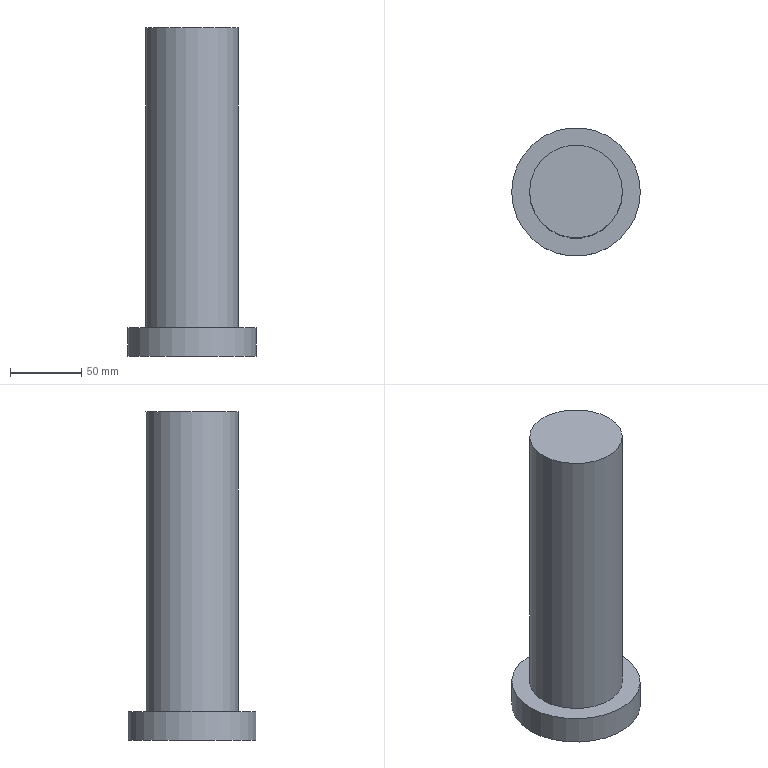Part | NX | features 平衡千斤顶缸销 2 | 1 solid | 5 faces | box 90 x 90 x 230 mm | volume 824079 mm3 | plane 3 | cylinder 2 | commonest cylinder face diameters 65 x1 90 x1
STEP:
#1=CARTESIAN_POINT('',(32.5,0.,210.));
#2=VERTEX_POINT('',#1);
#3=CARTESIAN_POINT('',(0.,0.,210.));
#4=DIRECTION('',(0.,0.,1.));
#5=DIRECTION('',(1.,0.,0.));
#6=AXIS2_PLACEMENT_3D('',#3,#4,#5);
#7=CIRCLE('',#6,32.5);
#8=EDGE_CURVE('',#2,#2,#7,.T.);
#9=ORIENTED_EDGE('',*,*,#8,.F.);
#10=EDGE_LOOP('',(#9));
#11=FACE_BOUND('',#10,.T.);
#12=CARTESIAN_POINT('',(-32.5,0.,0.));
#13=VERTEX_POINT('',#12);
#14=CARTESIAN_POINT('',(0.,0.,0.));
#15=DIRECTION('',(0.,0.,-1.));
#16=DIRECTION('',(-1.,0.,0.));
#17=AXIS2_PLACEMENT_3D('',#14,#15,#16);
#18=CIRCLE('',#17,32.5);
#19=EDGE_CURVE('',#13,#13,#18,.T.);
#20=ORIENTED_EDGE('',*,*,#19,.F.);
#21=EDGE_LOOP('',(#20));
#22=FACE_BOUND('',#21,.T.);
#23=CARTESIAN_POINT('',(0.,0.,210.));
#24=DIRECTION('',(0.,0.,-1.));
#25=DIRECTION('',(-1.,0.,0.));
#26=AXIS2_PLACEMENT_3D('',#23,#24,#25);
#27=CYLINDRICAL_SURFACE('',#26,32.5);
#28=ADVANCED_FACE('',(#11,#22),#27,.T.);
#29=ORIENTED_EDGE('',*,*,#8,.T.);
#30=EDGE_LOOP('',(#29));
#31=FACE_BOUND('',#30,.T.);
#32=CARTESIAN_POINT('',(0.,0.,210.));
#33=DIRECTION('',(0.,0.,1.));
#34=DIRECTION('',(1.,0.,0.));
#35=AXIS2_PLACEMENT_3D('',#32,#33,#34);
#36=PLANE('',#35);
#37=ADVANCED_FACE('',(#31),#36,.T.);
#38=CARTESIAN_POINT('',(-45.,0.,0.));
#39=VERTEX_POINT('',#38);
#40=CARTESIAN_POINT('',(0.,0.,0.));
#41=DIRECTION('',(0.,0.,-1.));
#42=DIRECTION('',(-1.,0.,0.));
#43=AXIS2_PLACEMENT_3D('',#40,#41,#42);
#44=CIRCLE('',#43,45.);
#45=EDGE_CURVE('',#39,#39,#44,.T.);
#46=ORIENTED_EDGE('',*,*,#45,.F.);
#47=EDGE_LOOP('',(#46));
#48=FACE_BOUND('',#47,.T.);
#49=ORIENTED_EDGE('',*,*,#19,.T.);
#50=EDGE_LOOP('',(#49));
#51=FACE_BOUND('',#50,.T.);
#52=CARTESIAN_POINT('',(0.,0.,0.));
#53=DIRECTION('',(0.,0.,-1.));
#54=DIRECTION('',(-1.,0.,0.));
#55=AXIS2_PLACEMENT_3D('',#52,#53,#54);
#56=PLANE('',#55);
#57=ADVANCED_FACE('',(#48,#51),#56,.F.);
#58=CARTESIAN_POINT('',(-45.,0.,-20.));
#59=VERTEX_POINT('',#58);
#60=CARTESIAN_POINT('',(0.,0.,-20.));
#61=DIRECTION('',(0.,0.,-1.));
#62=DIRECTION('',(-1.,0.,0.));
#63=AXIS2_PLACEMENT_3D('',#60,#61,#62);
#64=CIRCLE('',#63,45.);
#65=EDGE_CURVE('',#59,#59,#64,.T.);
#66=ORIENTED_EDGE('',*,*,#65,.F.);
#67=EDGE_LOOP('',(#66));
#68=FACE_BOUND('',#67,.T.);
#69=ORIENTED_EDGE('',*,*,#45,.T.);
#70=EDGE_LOOP('',(#69));
#71=FACE_BOUND('',#70,.T.);
#72=CARTESIAN_POINT('',(0.,0.,-20.));
#73=DIRECTION('',(0.,0.,1.));
#74=DIRECTION('',(1.,0.,0.));
#75=AXIS2_PLACEMENT_3D('',#72,#73,#74);
#76=CYLINDRICAL_SURFACE('',#75,45.);
#77=ADVANCED_FACE('',(#68,#71),#76,.T.);
#78=ORIENTED_EDGE('',*,*,#65,.T.);
#79=EDGE_LOOP('',(#78));
#80=FACE_BOUND('',#79,.T.);
#81=CARTESIAN_POINT('',(0.,0.,-20.));
#82=DIRECTION('',(0.,0.,-1.));
#83=DIRECTION('',(-1.,0.,0.));
#84=AXIS2_PLACEMENT_3D('',#81,#82,#83);
#85=PLANE('',#84);
#86=ADVANCED_FACE('',(#80),#85,.T.);
#87=CLOSED_SHELL('',(#28,#37,#57,#77,#86));
#88=MANIFOLD_SOLID_BREP('',#87);
#89=(LENGTH_UNIT()NAMED_UNIT(*)SI_UNIT(.MILLI.,.METRE.));
#90=UNCERTAINTY_MEASURE_WITH_UNIT(LENGTH_MEASURE(0.00001),#89,'','');
#91=(NAMED_UNIT(*)PLANE_ANGLE_UNIT()SI_UNIT($,.RADIAN.));
#92=(NAMED_UNIT(*)SI_UNIT($,.STERADIAN.)SOLID_ANGLE_UNIT());
#93=(GEOMETRIC_REPRESENTATION_CONTEXT(3)GLOBAL_UNCERTAINTY_ASSIGNED_CONTEXT((#90))GLOBAL_UNIT_ASSIGNED_CONTEXT((#89,#91,#92))REPRESENTATION_CONTEXT('',''));
#94=ADVANCED_BREP_SHAPE_REPRESENTATION('',(#88),#93);